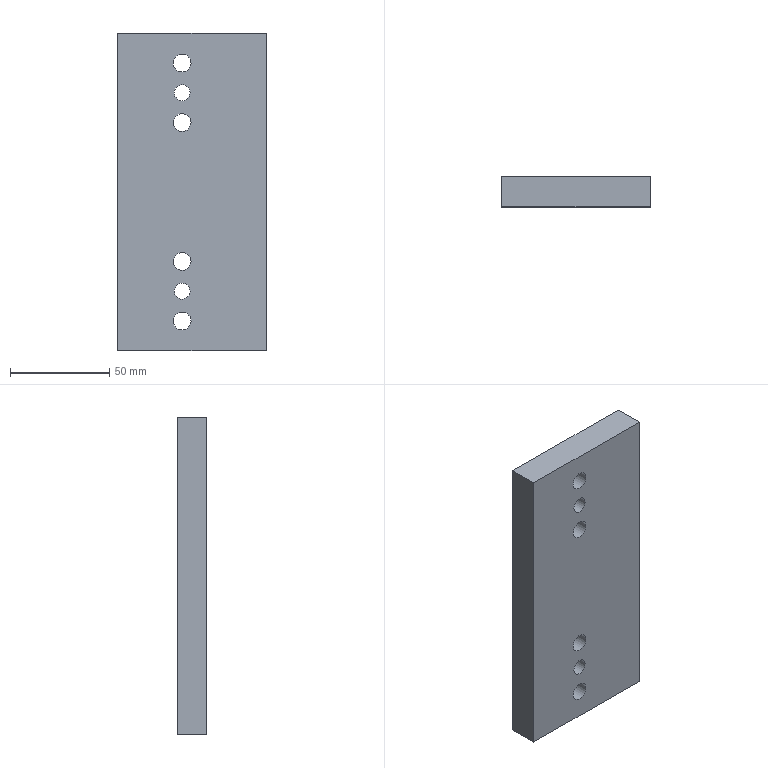Part | STEP file | SN10_008_007-02_PLACA | 1 solid | 12 faces | box 75 x 15 x 160 mm | volume 174675 mm3 | cylinder 6 | plane 6 | commonest cylinder face diameters 9 x4 8 x2
STEP:
#1=CARTESIAN_POINT('',(0.,0.,0.));
#2=DIRECTION('',(0.,0.,1.));
#3=DIRECTION('',(1.,0.,0.));
#4=AXIS2_PLACEMENT_3D('',#1,#2,#3);
#5=CARTESIAN_POINT('',(279.639,240.,404.352));
#6=VERTEX_POINT('',#5);
#7=CARTESIAN_POINT('',(276.129,240.,406.27));
#8=DIRECTION('',(0.,-1.,0.));
#9=DIRECTION('',(1.,0.,0.));
#10=AXIS2_PLACEMENT_3D('',#7,#8,#9);
#11=CIRCLE('',#10,4.);
#12=CARTESIAN_POINT('',(276.129,240.1,406.27));
#13=DIRECTION('',(0.,1.,0.));
#14=DIRECTION('',(0.8776,0.,-0.4794));
#15=AXIS2_PLACEMENT_3D('',#12,#13,#14);
#16=CYLINDRICAL_SURFACE('',#15,4.);
#17=CARTESIAN_POINT('',(12.066,-0.1));
#18=DIRECTION('',(-1.,0.));
#19=VECTOR('',#18,1.);
#20=LINE('',#17,#19);
#21=(GEOMETRIC_REPRESENTATION_CONTEXT(2)PARAMETRIC_REPRESENTATION_CONTEXT()REPRESENTATION_CONTEXT('',''));
#22=DEFINITIONAL_REPRESENTATION('',(#20),#21);
#23=PCURVE('',#16,#22);
#24=CARTESIAN_POINT('',(318.629,240.,446.));
#25=DIRECTION('',(0.,-1.,0.));
#26=DIRECTION('',(0.,0.,-1.));
#27=AXIS2_PLACEMENT_3D('',#24,#25,#26);
#28=PLANE('',#27);
#29=CARTESIAN_POINT('',(39.73,-42.5));
#30=DIRECTION('',(0.,1.));
#31=AXIS2_PLACEMENT_2D('',#29,#30);
#32=CIRCLE('',#31,4.);
#33=(GEOMETRIC_REPRESENTATION_CONTEXT(2)PARAMETRIC_REPRESENTATION_CONTEXT()REPRESENTATION_CONTEXT('',''));
#34=DEFINITIONAL_REPRESENTATION('',(#32),#33);
#35=PCURVE('',#28,#34);
#36=SURFACE_CURVE('',#11,(#23,#35),.PCURVE_S1.);
#37=EDGE_CURVE('',#6,#6,#36,.T.);
#38=ORIENTED_EDGE('',*,*,#37,.F.);
#39=CARTESIAN_POINT('',(279.639,255.,404.352));
#40=VERTEX_POINT('',#39);
#41=CARTESIAN_POINT('',(279.639,240.,404.352));
#42=CARTESIAN_POINT('',(279.639,255.,404.352));
#43=B_SPLINE_CURVE_WITH_KNOTS('',1,(#41,#42),.UNSPECIFIED.,.F.,.F.,(2,2),(-0.1,14.9),.PIECEWISE_BEZIER_KNOTS.);
#44=CARTESIAN_POINT('',(6.283,0.));
#45=DIRECTION('',(0.,1.));
#46=VECTOR('',#45,1.);
#47=LINE('',#44,#46);
#48=(GEOMETRIC_REPRESENTATION_CONTEXT(2)PARAMETRIC_REPRESENTATION_CONTEXT()REPRESENTATION_CONTEXT('',''));
#49=DEFINITIONAL_REPRESENTATION('',(#47),#48);
#50=PCURVE('',#16,#49);
#51=CARTESIAN_POINT('',(0.,0.));
#52=DIRECTION('',(0.,1.));
#53=VECTOR('',#52,1.);
#54=LINE('',#51,#53);
#55=(GEOMETRIC_REPRESENTATION_CONTEXT(2)PARAMETRIC_REPRESENTATION_CONTEXT()REPRESENTATION_CONTEXT('',''));
#56=DEFINITIONAL_REPRESENTATION('',(#54),#55);
#57=PCURVE('',#16,#56);
#58=SEAM_CURVE('',#43,(#50,#57),.PCURVE_S1.);
#59=EDGE_CURVE('',#6,#40,#58,.T.);
#60=ORIENTED_EDGE('',*,*,#59,.T.);
#61=CARTESIAN_POINT('',(276.129,255.,406.27));
#62=DIRECTION('',(0.,1.,0.));
#63=DIRECTION('',(1.,0.,0.));
#64=AXIS2_PLACEMENT_3D('',#61,#62,#63);
#65=CIRCLE('',#64,4.);
#66=CARTESIAN_POINT('',(-0.5,14.9));
#67=DIRECTION('',(1.,0.));
#68=VECTOR('',#67,1.);
#69=LINE('',#66,#68);
#70=(GEOMETRIC_REPRESENTATION_CONTEXT(2)PARAMETRIC_REPRESENTATION_CONTEXT()REPRESENTATION_CONTEXT('',''));
#71=DEFINITIONAL_REPRESENTATION('',(#69),#70);
#72=PCURVE('',#16,#71);
#73=CARTESIAN_POINT('',(243.629,255.,446.));
#74=DIRECTION('',(0.,1.,0.));
#75=DIRECTION('',(0.,0.,1.));
#76=AXIS2_PLACEMENT_3D('',#73,#74,#75);
#77=PLANE('',#76);
#78=CARTESIAN_POINT('',(-39.73,32.5));
#79=DIRECTION('',(0.,1.));
#80=AXIS2_PLACEMENT_2D('',#78,#79);
#81=CIRCLE('',#80,4.);
#82=(GEOMETRIC_REPRESENTATION_CONTEXT(2)PARAMETRIC_REPRESENTATION_CONTEXT()REPRESENTATION_CONTEXT('',''));
#83=DEFINITIONAL_REPRESENTATION('',(#81),#82);
#84=PCURVE('',#77,#83);
#85=SURFACE_CURVE('',#65,(#72,#84),.PCURVE_S1.);
#86=EDGE_CURVE('',#40,#40,#85,.T.);
#87=ORIENTED_EDGE('',*,*,#86,.F.);
#88=ORIENTED_EDGE('',*,*,#59,.F.);
#89=EDGE_LOOP('',(#38,#60,#87,#88));
#90=FACE_BOUND('',#89,.F.);
#91=ADVANCED_FACE('',(#90),#16,.F.);
#92=CARTESIAN_POINT('',(243.629,240.,436.27));
#93=VERTEX_POINT('',#92);
#94=CARTESIAN_POINT('',(243.629,240.,276.27));
#95=VERTEX_POINT('',#94);
#96=CARTESIAN_POINT('',(243.629,240.,436.27));
#97=DIRECTION('',(0.,0.,-1.));
#98=VECTOR('',#97,1.);
#99=LINE('',#96,#98);
#100=CARTESIAN_POINT('',(9.73,-75.));
#101=DIRECTION('',(1.,0.));
#102=VECTOR('',#101,1.);
#103=LINE('',#100,#102);
#104=(GEOMETRIC_REPRESENTATION_CONTEXT(2)PARAMETRIC_REPRESENTATION_CONTEXT()REPRESENTATION_CONTEXT('',''));
#105=DEFINITIONAL_REPRESENTATION('',(#103),#104);
#106=PCURVE('',#28,#105);
#107=CARTESIAN_POINT('',(243.629,255.,446.));
#108=DIRECTION('',(1.,0.,0.));
#109=DIRECTION('',(0.,0.,-1.));
#110=AXIS2_PLACEMENT_3D('',#107,#108,#109);
#111=PLANE('',#110);
#112=CARTESIAN_POINT('',(9.73,-15.));
#113=DIRECTION('',(1.,0.));
#114=VECTOR('',#113,1.);
#115=LINE('',#112,#114);
#116=(GEOMETRIC_REPRESENTATION_CONTEXT(2)PARAMETRIC_REPRESENTATION_CONTEXT()REPRESENTATION_CONTEXT('',''));
#117=DEFINITIONAL_REPRESENTATION('',(#115),#116);
#118=PCURVE('',#111,#117);
#119=SURFACE_CURVE('',#99,(#106,#118),.PCURVE_S1.);
#120=EDGE_CURVE('',#93,#95,#119,.T.);
#121=ORIENTED_EDGE('',*,*,#120,.T.);
#122=CARTESIAN_POINT('',(318.629,240.,276.27));
#123=VERTEX_POINT('',#122);
#124=CARTESIAN_POINT('',(318.629,240.,276.27));
#125=DIRECTION('',(-1.,0.,0.));
#126=VECTOR('',#125,1.);
#127=LINE('',#124,#126);
#128=CARTESIAN_POINT('',(169.73,0.));
#129=DIRECTION('',(0.,-1.));
#130=VECTOR('',#129,1.);
#131=LINE('',#128,#130);
#132=(GEOMETRIC_REPRESENTATION_CONTEXT(2)PARAMETRIC_REPRESENTATION_CONTEXT()REPRESENTATION_CONTEXT('',''));
#133=DEFINITIONAL_REPRESENTATION('',(#131),#132);
#134=PCURVE('',#28,#133);
#135=CARTESIAN_POINT('',(243.629,270.,276.27));
#136=DIRECTION('',(0.,0.,-1.));
#137=DIRECTION('',(-1.,0.,0.));
#138=AXIS2_PLACEMENT_3D('',#135,#136,#137);
#139=PLANE('',#138);
#140=CARTESIAN_POINT('',(-75.,-30.));
#141=DIRECTION('',(1.,0.));
#142=VECTOR('',#141,1.);
#143=LINE('',#140,#142);
#144=(GEOMETRIC_REPRESENTATION_CONTEXT(2)PARAMETRIC_REPRESENTATION_CONTEXT()REPRESENTATION_CONTEXT('',''));
#145=DEFINITIONAL_REPRESENTATION('',(#143),#144);
#146=PCURVE('',#139,#145);
#147=SURFACE_CURVE('',#127,(#134,#146),.PCURVE_S1.);
#148=EDGE_CURVE('',#123,#95,#147,.T.);
#149=ORIENTED_EDGE('',*,*,#148,.F.);
#150=CARTESIAN_POINT('',(318.629,240.,436.27));
#151=VERTEX_POINT('',#150);
#152=CARTESIAN_POINT('',(318.629,240.,436.27));
#153=DIRECTION('',(0.,0.,-1.));
#154=VECTOR('',#153,1.);
#155=LINE('',#152,#154);
#156=CARTESIAN_POINT('',(9.73,0.));
#157=DIRECTION('',(1.,0.));
#158=VECTOR('',#157,1.);
#159=LINE('',#156,#158);
#160=(GEOMETRIC_REPRESENTATION_CONTEXT(2)PARAMETRIC_REPRESENTATION_CONTEXT()REPRESENTATION_CONTEXT('',''));
#161=DEFINITIONAL_REPRESENTATION('',(#159),#160);
#162=PCURVE('',#28,#161);
#163=CARTESIAN_POINT('',(318.629,240.,446.));
#164=DIRECTION('',(-1.,0.,0.));
#165=DIRECTION('',(0.,0.,1.));
#166=AXIS2_PLACEMENT_3D('',#163,#164,#165);
#167=PLANE('',#166);
#168=CARTESIAN_POINT('',(-9.73,0.));
#169=DIRECTION('',(-1.,0.));
#170=VECTOR('',#169,1.);
#171=LINE('',#168,#170);
#172=(GEOMETRIC_REPRESENTATION_CONTEXT(2)PARAMETRIC_REPRESENTATION_CONTEXT()REPRESENTATION_CONTEXT('',''));
#173=DEFINITIONAL_REPRESENTATION('',(#171),#172);
#174=PCURVE('',#167,#173);
#175=SURFACE_CURVE('',#155,(#162,#174),.PCURVE_S1.);
#176=EDGE_CURVE('',#151,#123,#175,.T.);
#177=ORIENTED_EDGE('',*,*,#176,.F.);
#178=CARTESIAN_POINT('',(243.629,240.,436.27));
#179=DIRECTION('',(1.,0.,0.));
#180=VECTOR('',#179,1.);
#181=LINE('',#178,#180);
#182=CARTESIAN_POINT('',(9.73,-75.));
#183=DIRECTION('',(0.,1.));
#184=VECTOR('',#183,1.);
#185=LINE('',#182,#184);
#186=(GEOMETRIC_REPRESENTATION_CONTEXT(2)PARAMETRIC_REPRESENTATION_CONTEXT()REPRESENTATION_CONTEXT('',''));
#187=DEFINITIONAL_REPRESENTATION('',(#185),#186);
#188=PCURVE('',#28,#187);
#189=CARTESIAN_POINT('',(243.629,255.,436.27));
#190=DIRECTION('',(0.,0.,1.));
#191=DIRECTION('',(1.,0.,0.));
#192=AXIS2_PLACEMENT_3D('',#189,#190,#191);
#193=PLANE('',#192);
#194=CARTESIAN_POINT('',(0.,-15.));
#195=DIRECTION('',(1.,0.));
#196=VECTOR('',#195,1.);
#197=LINE('',#194,#196);
#198=(GEOMETRIC_REPRESENTATION_CONTEXT(2)PARAMETRIC_REPRESENTATION_CONTEXT()REPRESENTATION_CONTEXT('',''));
#199=DEFINITIONAL_REPRESENTATION('',(#197),#198);
#200=PCURVE('',#193,#199);
#201=SURFACE_CURVE('',#181,(#188,#200),.PCURVE_S1.);
#202=EDGE_CURVE('',#93,#151,#201,.T.);
#203=ORIENTED_EDGE('',*,*,#202,.F.);
#204=EDGE_LOOP('',(#121,#149,#177,#203));
#205=FACE_BOUND('',#204,.T.);
#206=ORIENTED_EDGE('',*,*,#37,.F.);
#207=EDGE_LOOP('',(#206));
#208=FACE_BOUND('',#207,.T.);
#209=CARTESIAN_POINT('',(279.639,240.,304.352));
#210=VERTEX_POINT('',#209);
#211=CARTESIAN_POINT('',(276.129,240.,306.27));
#212=DIRECTION('',(0.,-1.,0.));
#213=DIRECTION('',(1.,0.,0.));
#214=AXIS2_PLACEMENT_3D('',#211,#212,#213);
#215=CIRCLE('',#214,4.);
#216=CARTESIAN_POINT('',(139.73,-42.5));
#217=DIRECTION('',(0.,1.));
#218=AXIS2_PLACEMENT_2D('',#216,#217);
#219=CIRCLE('',#218,4.);
#220=(GEOMETRIC_REPRESENTATION_CONTEXT(2)PARAMETRIC_REPRESENTATION_CONTEXT()REPRESENTATION_CONTEXT('',''));
#221=DEFINITIONAL_REPRESENTATION('',(#219),#220);
#222=PCURVE('',#28,#221);
#223=CARTESIAN_POINT('',(276.129,240.1,306.27));
#224=DIRECTION('',(0.,1.,0.));
#225=DIRECTION('',(0.8776,0.,-0.4794));
#226=AXIS2_PLACEMENT_3D('',#223,#224,#225);
#227=CYLINDRICAL_SURFACE('',#226,4.);
#228=CARTESIAN_POINT('',(12.066,-0.1));
#229=DIRECTION('',(-1.,0.));
#230=VECTOR('',#229,1.);
#231=LINE('',#228,#230);
#232=(GEOMETRIC_REPRESENTATION_CONTEXT(2)PARAMETRIC_REPRESENTATION_CONTEXT()REPRESENTATION_CONTEXT('',''));
#233=DEFINITIONAL_REPRESENTATION('',(#231),#232);
#234=PCURVE('',#227,#233);
#235=SURFACE_CURVE('',#215,(#222,#234),.PCURVE_S1.);
#236=EDGE_CURVE('',#210,#210,#235,.T.);
#237=ORIENTED_EDGE('',*,*,#236,.F.);
#238=EDGE_LOOP('',(#237));
#239=FACE_BOUND('',#238,.T.);
#240=CARTESIAN_POINT('',(280.078,240.,319.113));
#241=VERTEX_POINT('',#240);
#242=CARTESIAN_POINT('',(276.129,240.,321.27));
#243=DIRECTION('',(0.,-1.,0.));
#244=DIRECTION('',(1.,0.,0.));
#245=AXIS2_PLACEMENT_3D('',#242,#243,#244);
#246=CIRCLE('',#245,4.5);
#247=CARTESIAN_POINT('',(124.73,-42.5));
#248=DIRECTION('',(0.,1.));
#249=AXIS2_PLACEMENT_2D('',#247,#248);
#250=CIRCLE('',#249,4.5);
#251=(GEOMETRIC_REPRESENTATION_CONTEXT(2)PARAMETRIC_REPRESENTATION_CONTEXT()REPRESENTATION_CONTEXT('',''));
#252=DEFINITIONAL_REPRESENTATION('',(#250),#251);
#253=PCURVE('',#28,#252);
#254=CARTESIAN_POINT('',(276.129,240.1,321.27));
#255=DIRECTION('',(0.,1.,0.));
#256=DIRECTION('',(0.8776,0.,-0.4794));
#257=AXIS2_PLACEMENT_3D('',#254,#255,#256);
#258=CYLINDRICAL_SURFACE('',#257,4.5);
#259=CARTESIAN_POINT('',(12.066,-0.1));
#260=DIRECTION('',(-1.,0.));
#261=VECTOR('',#260,1.);
#262=LINE('',#259,#261);
#263=(GEOMETRIC_REPRESENTATION_CONTEXT(2)PARAMETRIC_REPRESENTATION_CONTEXT()REPRESENTATION_CONTEXT('',''));
#264=DEFINITIONAL_REPRESENTATION('',(#262),#263);
#265=PCURVE('',#258,#264);
#266=SURFACE_CURVE('',#246,(#253,#265),.PCURVE_S1.);
#267=EDGE_CURVE('',#241,#241,#266,.T.);
#268=ORIENTED_EDGE('',*,*,#267,.F.);
#269=EDGE_LOOP('',(#268));
#270=FACE_BOUND('',#269,.T.);
#271=CARTESIAN_POINT('',(280.078,240.,289.113));
#272=VERTEX_POINT('',#271);
#273=CARTESIAN_POINT('',(276.129,240.,291.27));
#274=DIRECTION('',(0.,-1.,0.));
#275=DIRECTION('',(1.,0.,0.));
#276=AXIS2_PLACEMENT_3D('',#273,#274,#275);
#277=CIRCLE('',#276,4.5);
#278=CARTESIAN_POINT('',(154.73,-42.5));
#279=DIRECTION('',(0.,1.));
#280=AXIS2_PLACEMENT_2D('',#278,#279);
#281=CIRCLE('',#280,4.5);
#282=(GEOMETRIC_REPRESENTATION_CONTEXT(2)PARAMETRIC_REPRESENTATION_CONTEXT()REPRESENTATION_CONTEXT('',''));
#283=DEFINITIONAL_REPRESENTATION('',(#281),#282);
#284=PCURVE('',#28,#283);
#285=CARTESIAN_POINT('',(276.129,240.1,291.27));
#286=DIRECTION('',(0.,1.,0.));
#287=DIRECTION('',(0.8776,0.,-0.4794));
#288=AXIS2_PLACEMENT_3D('',#285,#286,#287);
#289=CYLINDRICAL_SURFACE('',#288,4.5);
#290=CARTESIAN_POINT('',(12.066,-0.1));
#291=DIRECTION('',(-1.,0.));
#292=VECTOR('',#291,1.);
#293=LINE('',#290,#292);
#294=(GEOMETRIC_REPRESENTATION_CONTEXT(2)PARAMETRIC_REPRESENTATION_CONTEXT()REPRESENTATION_CONTEXT('',''));
#295=DEFINITIONAL_REPRESENTATION('',(#293),#294);
#296=PCURVE('',#289,#295);
#297=SURFACE_CURVE('',#277,(#284,#296),.PCURVE_S1.);
#298=EDGE_CURVE('',#272,#272,#297,.T.);
#299=ORIENTED_EDGE('',*,*,#298,.F.);
#300=EDGE_LOOP('',(#299));
#301=FACE_BOUND('',#300,.T.);
#302=CARTESIAN_POINT('',(280.078,240.,389.113));
#303=VERTEX_POINT('',#302);
#304=CARTESIAN_POINT('',(276.129,240.,391.27));
#305=DIRECTION('',(0.,-1.,0.));
#306=DIRECTION('',(1.,0.,0.));
#307=AXIS2_PLACEMENT_3D('',#304,#305,#306);
#308=CIRCLE('',#307,4.5);
#309=CARTESIAN_POINT('',(54.73,-42.5));
#310=DIRECTION('',(0.,1.));
#311=AXIS2_PLACEMENT_2D('',#309,#310);
#312=CIRCLE('',#311,4.5);
#313=(GEOMETRIC_REPRESENTATION_CONTEXT(2)PARAMETRIC_REPRESENTATION_CONTEXT()REPRESENTATION_CONTEXT('',''));
#314=DEFINITIONAL_REPRESENTATION('',(#312),#313);
#315=PCURVE('',#28,#314);
#316=CARTESIAN_POINT('',(276.129,240.1,391.27));
#317=DIRECTION('',(0.,1.,0.));
#318=DIRECTION('',(0.8776,0.,-0.4794));
#319=AXIS2_PLACEMENT_3D('',#316,#317,#318);
#320=CYLINDRICAL_SURFACE('',#319,4.5);
#321=CARTESIAN_POINT('',(12.066,-0.1));
#322=DIRECTION('',(-1.,0.));
#323=VECTOR('',#322,1.);
#324=LINE('',#321,#323);
#325=(GEOMETRIC_REPRESENTATION_CONTEXT(2)PARAMETRIC_REPRESENTATION_CONTEXT()REPRESENTATION_CONTEXT('',''));
#326=DEFINITIONAL_REPRESENTATION('',(#324),#325);
#327=PCURVE('',#320,#326);
#328=SURFACE_CURVE('',#308,(#315,#327),.PCURVE_S1.);
#329=EDGE_CURVE('',#303,#303,#328,.T.);
#330=ORIENTED_EDGE('',*,*,#329,.F.);
#331=EDGE_LOOP('',(#330));
#332=FACE_BOUND('',#331,.T.);
#333=CARTESIAN_POINT('',(280.078,240.,419.113));
#334=VERTEX_POINT('',#333);
#335=CARTESIAN_POINT('',(276.129,240.,421.27));
#336=DIRECTION('',(0.,-1.,0.));
#337=DIRECTION('',(1.,0.,0.));
#338=AXIS2_PLACEMENT_3D('',#335,#336,#337);
#339=CIRCLE('',#338,4.5);
#340=CARTESIAN_POINT('',(24.73,-42.5));
#341=DIRECTION('',(0.,1.));
#342=AXIS2_PLACEMENT_2D('',#340,#341);
#343=CIRCLE('',#342,4.5);
#344=(GEOMETRIC_REPRESENTATION_CONTEXT(2)PARAMETRIC_REPRESENTATION_CONTEXT()REPRESENTATION_CONTEXT('',''));
#345=DEFINITIONAL_REPRESENTATION('',(#343),#344);
#346=PCURVE('',#28,#345);
#347=CARTESIAN_POINT('',(276.129,240.1,421.27));
#348=DIRECTION('',(0.,1.,0.));
#349=DIRECTION('',(0.8776,0.,-0.4794));
#350=AXIS2_PLACEMENT_3D('',#347,#348,#349);
#351=CYLINDRICAL_SURFACE('',#350,4.5);
#352=CARTESIAN_POINT('',(12.066,-0.1));
#353=DIRECTION('',(-1.,0.));
#354=VECTOR('',#353,1.);
#355=LINE('',#352,#354);
#356=(GEOMETRIC_REPRESENTATION_CONTEXT(2)PARAMETRIC_REPRESENTATION_CONTEXT()REPRESENTATION_CONTEXT('',''));
#357=DEFINITIONAL_REPRESENTATION('',(#355),#356);
#358=PCURVE('',#351,#357);
#359=SURFACE_CURVE('',#339,(#346,#358),.PCURVE_S1.);
#360=EDGE_CURVE('',#334,#334,#359,.T.);
#361=ORIENTED_EDGE('',*,*,#360,.F.);
#362=EDGE_LOOP('',(#361));
#363=FACE_BOUND('',#362,.T.);
#364=ADVANCED_FACE('',(#205,#208,#239,#270,#301,#332,#363),#28,.T.);
#365=CARTESIAN_POINT('',(318.629,255.,436.27));
#366=VERTEX_POINT('',#365);
#367=CARTESIAN_POINT('',(318.629,255.,276.27));
#368=VERTEX_POINT('',#367);
#369=CARTESIAN_POINT('',(318.629,255.,436.27));
#370=DIRECTION('',(0.,0.,-1.));
#371=VECTOR('',#370,1.);
#372=LINE('',#369,#371);
#373=CARTESIAN_POINT('',(-9.73,75.));
#374=DIRECTION('',(-1.,0.));
#375=VECTOR('',#374,1.);
#376=LINE('',#373,#375);
#377=(GEOMETRIC_REPRESENTATION_CONTEXT(2)PARAMETRIC_REPRESENTATION_CONTEXT()REPRESENTATION_CONTEXT('',''));
#378=DEFINITIONAL_REPRESENTATION('',(#376),#377);
#379=PCURVE('',#77,#378);
#380=CARTESIAN_POINT('',(-9.73,15.));
#381=DIRECTION('',(-1.,0.));
#382=VECTOR('',#381,1.);
#383=LINE('',#380,#382);
#384=(GEOMETRIC_REPRESENTATION_CONTEXT(2)PARAMETRIC_REPRESENTATION_CONTEXT()REPRESENTATION_CONTEXT('',''));
#385=DEFINITIONAL_REPRESENTATION('',(#383),#384);
#386=PCURVE('',#167,#385);
#387=SURFACE_CURVE('',#372,(#379,#386),.PCURVE_S1.);
#388=EDGE_CURVE('',#366,#368,#387,.T.);
#389=ORIENTED_EDGE('',*,*,#388,.T.);
#390=CARTESIAN_POINT('',(243.629,255.,276.27));
#391=VERTEX_POINT('',#390);
#392=CARTESIAN_POINT('',(243.629,255.,276.27));
#393=DIRECTION('',(1.,0.,0.));
#394=VECTOR('',#393,1.);
#395=LINE('',#392,#394);
#396=CARTESIAN_POINT('',(-169.73,0.));
#397=DIRECTION('',(0.,1.));
#398=VECTOR('',#397,1.);
#399=LINE('',#396,#398);
#400=(GEOMETRIC_REPRESENTATION_CONTEXT(2)PARAMETRIC_REPRESENTATION_CONTEXT()REPRESENTATION_CONTEXT('',''));
#401=DEFINITIONAL_REPRESENTATION('',(#399),#400);
#402=PCURVE('',#77,#401);
#403=CARTESIAN_POINT('',(0.,-15.));
#404=DIRECTION('',(-1.,0.));
#405=VECTOR('',#404,1.);
#406=LINE('',#403,#405);
#407=(GEOMETRIC_REPRESENTATION_CONTEXT(2)PARAMETRIC_REPRESENTATION_CONTEXT()REPRESENTATION_CONTEXT('',''));
#408=DEFINITIONAL_REPRESENTATION('',(#406),#407);
#409=PCURVE('',#139,#408);
#410=SURFACE_CURVE('',#395,(#402,#409),.PCURVE_S1.);
#411=EDGE_CURVE('',#391,#368,#410,.T.);
#412=ORIENTED_EDGE('',*,*,#411,.F.);
#413=CARTESIAN_POINT('',(243.629,255.,436.27));
#414=VERTEX_POINT('',#413);
#415=CARTESIAN_POINT('',(243.629,255.,436.27));
#416=DIRECTION('',(0.,0.,-1.));
#417=VECTOR('',#416,1.);
#418=LINE('',#415,#417);
#419=CARTESIAN_POINT('',(-9.73,0.));
#420=DIRECTION('',(-1.,0.));
#421=VECTOR('',#420,1.);
#422=LINE('',#419,#421);
#423=(GEOMETRIC_REPRESENTATION_CONTEXT(2)PARAMETRIC_REPRESENTATION_CONTEXT()REPRESENTATION_CONTEXT('',''));
#424=DEFINITIONAL_REPRESENTATION('',(#422),#423);
#425=PCURVE('',#77,#424);
#426=CARTESIAN_POINT('',(9.73,0.));
#427=DIRECTION('',(1.,0.));
#428=VECTOR('',#427,1.);
#429=LINE('',#426,#428);
#430=(GEOMETRIC_REPRESENTATION_CONTEXT(2)PARAMETRIC_REPRESENTATION_CONTEXT()REPRESENTATION_CONTEXT('',''));
#431=DEFINITIONAL_REPRESENTATION('',(#429),#430);
#432=PCURVE('',#111,#431);
#433=SURFACE_CURVE('',#418,(#425,#432),.PCURVE_S1.);
#434=EDGE_CURVE('',#414,#391,#433,.T.);
#435=ORIENTED_EDGE('',*,*,#434,.F.);
#436=CARTESIAN_POINT('',(243.629,255.,436.27));
#437=DIRECTION('',(1.,0.,0.));
#438=VECTOR('',#437,1.);
#439=LINE('',#436,#438);
#440=CARTESIAN_POINT('',(-9.73,0.));
#441=DIRECTION('',(0.,1.));
#442=VECTOR('',#441,1.);
#443=LINE('',#440,#442);
#444=(GEOMETRIC_REPRESENTATION_CONTEXT(2)PARAMETRIC_REPRESENTATION_CONTEXT()REPRESENTATION_CONTEXT('',''));
#445=DEFINITIONAL_REPRESENTATION('',(#443),#444);
#446=PCURVE('',#77,#445);
#447=CARTESIAN_POINT('',(0.,0.));
#448=DIRECTION('',(1.,0.));
#449=VECTOR('',#448,1.);
#450=LINE('',#447,#449);
#451=(GEOMETRIC_REPRESENTATION_CONTEXT(2)PARAMETRIC_REPRESENTATION_CONTEXT()REPRESENTATION_CONTEXT('',''));
#452=DEFINITIONAL_REPRESENTATION('',(#450),#451);
#453=PCURVE('',#193,#452);
#454=SURFACE_CURVE('',#439,(#446,#453),.PCURVE_S1.);
#455=EDGE_CURVE('',#414,#366,#454,.T.);
#456=ORIENTED_EDGE('',*,*,#455,.T.);
#457=EDGE_LOOP('',(#389,#412,#435,#456));
#458=FACE_BOUND('',#457,.T.);
#459=ORIENTED_EDGE('',*,*,#86,.F.);
#460=EDGE_LOOP('',(#459));
#461=FACE_BOUND('',#460,.T.);
#462=CARTESIAN_POINT('',(279.639,255.,304.352));
#463=VERTEX_POINT('',#462);
#464=CARTESIAN_POINT('',(276.129,255.,306.27));
#465=DIRECTION('',(0.,1.,0.));
#466=DIRECTION('',(1.,0.,0.));
#467=AXIS2_PLACEMENT_3D('',#464,#465,#466);
#468=CIRCLE('',#467,4.);
#469=CARTESIAN_POINT('',(-139.73,32.5));
#470=DIRECTION('',(0.,1.));
#471=AXIS2_PLACEMENT_2D('',#469,#470);
#472=CIRCLE('',#471,4.);
#473=(GEOMETRIC_REPRESENTATION_CONTEXT(2)PARAMETRIC_REPRESENTATION_CONTEXT()REPRESENTATION_CONTEXT('',''));
#474=DEFINITIONAL_REPRESENTATION('',(#472),#473);
#475=PCURVE('',#77,#474);
#476=CARTESIAN_POINT('',(-0.5,14.9));
#477=DIRECTION('',(1.,0.));
#478=VECTOR('',#477,1.);
#479=LINE('',#476,#478);
#480=(GEOMETRIC_REPRESENTATION_CONTEXT(2)PARAMETRIC_REPRESENTATION_CONTEXT()REPRESENTATION_CONTEXT('',''));
#481=DEFINITIONAL_REPRESENTATION('',(#479),#480);
#482=PCURVE('',#227,#481);
#483=SURFACE_CURVE('',#468,(#475,#482),.PCURVE_S1.);
#484=EDGE_CURVE('',#463,#463,#483,.T.);
#485=ORIENTED_EDGE('',*,*,#484,.F.);
#486=EDGE_LOOP('',(#485));
#487=FACE_BOUND('',#486,.T.);
#488=CARTESIAN_POINT('',(280.078,255.,319.113));
#489=VERTEX_POINT('',#488);
#490=CARTESIAN_POINT('',(276.129,255.,321.27));
#491=DIRECTION('',(0.,1.,0.));
#492=DIRECTION('',(1.,0.,0.));
#493=AXIS2_PLACEMENT_3D('',#490,#491,#492);
#494=CIRCLE('',#493,4.5);
#495=CARTESIAN_POINT('',(-124.73,32.5));
#496=DIRECTION('',(0.,1.));
#497=AXIS2_PLACEMENT_2D('',#495,#496);
#498=CIRCLE('',#497,4.5);
#499=(GEOMETRIC_REPRESENTATION_CONTEXT(2)PARAMETRIC_REPRESENTATION_CONTEXT()REPRESENTATION_CONTEXT('',''));
#500=DEFINITIONAL_REPRESENTATION('',(#498),#499);
#501=PCURVE('',#77,#500);
#502=CARTESIAN_POINT('',(-0.5,14.9));
#503=DIRECTION('',(1.,0.));
#504=VECTOR('',#503,1.);
#505=LINE('',#502,#504);
#506=(GEOMETRIC_REPRESENTATION_CONTEXT(2)PARAMETRIC_REPRESENTATION_CONTEXT()REPRESENTATION_CONTEXT('',''));
#507=DEFINITIONAL_REPRESENTATION('',(#505),#506);
#508=PCURVE('',#258,#507);
#509=SURFACE_CURVE('',#494,(#501,#508),.PCURVE_S1.);
#510=EDGE_CURVE('',#489,#489,#509,.T.);
#511=ORIENTED_EDGE('',*,*,#510,.F.);
#512=EDGE_LOOP('',(#511));
#513=FACE_BOUND('',#512,.T.);
#514=CARTESIAN_POINT('',(280.078,255.,289.113));
#515=VERTEX_POINT('',#514);
#516=CARTESIAN_POINT('',(276.129,255.,291.27));
#517=DIRECTION('',(0.,1.,0.));
#518=DIRECTION('',(1.,0.,0.));
#519=AXIS2_PLACEMENT_3D('',#516,#517,#518);
#520=CIRCLE('',#519,4.5);
#521=CARTESIAN_POINT('',(-154.73,32.5));
#522=DIRECTION('',(0.,1.));
#523=AXIS2_PLACEMENT_2D('',#521,#522);
#524=CIRCLE('',#523,4.5);
#525=(GEOMETRIC_REPRESENTATION_CONTEXT(2)PARAMETRIC_REPRESENTATION_CONTEXT()REPRESENTATION_CONTEXT('',''));
#526=DEFINITIONAL_REPRESENTATION('',(#524),#525);
#527=PCURVE('',#77,#526);
#528=CARTESIAN_POINT('',(-0.5,14.9));
#529=DIRECTION('',(1.,0.));
#530=VECTOR('',#529,1.);
#531=LINE('',#528,#530);
#532=(GEOMETRIC_REPRESENTATION_CONTEXT(2)PARAMETRIC_REPRESENTATION_CONTEXT()REPRESENTATION_CONTEXT('',''));
#533=DEFINITIONAL_REPRESENTATION('',(#531),#532);
#534=PCURVE('',#289,#533);
#535=SURFACE_CURVE('',#520,(#527,#534),.PCURVE_S1.);
#536=EDGE_CURVE('',#515,#515,#535,.T.);
#537=ORIENTED_EDGE('',*,*,#536,.F.);
#538=EDGE_LOOP('',(#537));
#539=FACE_BOUND('',#538,.T.);
#540=CARTESIAN_POINT('',(280.078,255.,389.113));
#541=VERTEX_POINT('',#540);
#542=CARTESIAN_POINT('',(276.129,255.,391.27));
#543=DIRECTION('',(0.,1.,0.));
#544=DIRECTION('',(1.,0.,0.));
#545=AXIS2_PLACEMENT_3D('',#542,#543,#544);
#546=CIRCLE('',#545,4.5);
#547=CARTESIAN_POINT('',(-54.73,32.5));
#548=DIRECTION('',(0.,1.));
#549=AXIS2_PLACEMENT_2D('',#547,#548);
#550=CIRCLE('',#549,4.5);
#551=(GEOMETRIC_REPRESENTATION_CONTEXT(2)PARAMETRIC_REPRESENTATION_CONTEXT()REPRESENTATION_CONTEXT('',''));
#552=DEFINITIONAL_REPRESENTATION('',(#550),#551);
#553=PCURVE('',#77,#552);
#554=CARTESIAN_POINT('',(-0.5,14.9));
#555=DIRECTION('',(1.,0.));
#556=VECTOR('',#555,1.);
#557=LINE('',#554,#556);
#558=(GEOMETRIC_REPRESENTATION_CONTEXT(2)PARAMETRIC_REPRESENTATION_CONTEXT()REPRESENTATION_CONTEXT('',''));
#559=DEFINITIONAL_REPRESENTATION('',(#557),#558);
#560=PCURVE('',#320,#559);
#561=SURFACE_CURVE('',#546,(#553,#560),.PCURVE_S1.);
#562=EDGE_CURVE('',#541,#541,#561,.T.);
#563=ORIENTED_EDGE('',*,*,#562,.F.);
#564=EDGE_LOOP('',(#563));
#565=FACE_BOUND('',#564,.T.);
#566=CARTESIAN_POINT('',(280.078,255.,419.113));
#567=VERTEX_POINT('',#566);
#568=CARTESIAN_POINT('',(276.129,255.,421.27));
#569=DIRECTION('',(0.,1.,0.));
#570=DIRECTION('',(1.,0.,0.));
#571=AXIS2_PLACEMENT_3D('',#568,#569,#570);
#572=CIRCLE('',#571,4.5);
#573=CARTESIAN_POINT('',(-24.73,32.5));
#574=DIRECTION('',(0.,1.));
#575=AXIS2_PLACEMENT_2D('',#573,#574);
#576=CIRCLE('',#575,4.5);
#577=(GEOMETRIC_REPRESENTATION_CONTEXT(2)PARAMETRIC_REPRESENTATION_CONTEXT()REPRESENTATION_CONTEXT('',''));
#578=DEFINITIONAL_REPRESENTATION('',(#576),#577);
#579=PCURVE('',#77,#578);
#580=CARTESIAN_POINT('',(-0.5,14.9));
#581=DIRECTION('',(1.,0.));
#582=VECTOR('',#581,1.);
#583=LINE('',#580,#582);
#584=(GEOMETRIC_REPRESENTATION_CONTEXT(2)PARAMETRIC_REPRESENTATION_CONTEXT()REPRESENTATION_CONTEXT('',''));
#585=DEFINITIONAL_REPRESENTATION('',(#583),#584);
#586=PCURVE('',#351,#585);
#587=SURFACE_CURVE('',#572,(#579,#586),.PCURVE_S1.);
#588=EDGE_CURVE('',#567,#567,#587,.T.);
#589=ORIENTED_EDGE('',*,*,#588,.F.);
#590=EDGE_LOOP('',(#589));
#591=FACE_BOUND('',#590,.T.);
#592=ADVANCED_FACE('',(#458,#461,#487,#513,#539,#565,#591),#77,.T.);
#593=CARTESIAN_POINT('',(243.629,255.,436.27));
#594=DIRECTION('',(0.,-1.,0.));
#595=VECTOR('',#594,1.);
#596=LINE('',#593,#595);
#597=CARTESIAN_POINT('',(9.73,0.));
#598=DIRECTION('',(0.,-1.));
#599=VECTOR('',#598,1.);
#600=LINE('',#597,#599);
#601=(GEOMETRIC_REPRESENTATION_CONTEXT(2)PARAMETRIC_REPRESENTATION_CONTEXT()REPRESENTATION_CONTEXT('',''));
#602=DEFINITIONAL_REPRESENTATION('',(#600),#601);
#603=PCURVE('',#111,#602);
#604=CARTESIAN_POINT('',(0.,0.));
#605=DIRECTION('',(0.,-1.));
#606=VECTOR('',#605,1.);
#607=LINE('',#604,#606);
#608=(GEOMETRIC_REPRESENTATION_CONTEXT(2)PARAMETRIC_REPRESENTATION_CONTEXT()REPRESENTATION_CONTEXT('',''));
#609=DEFINITIONAL_REPRESENTATION('',(#607),#608);
#610=PCURVE('',#193,#609);
#611=SURFACE_CURVE('',#596,(#603,#610),.PCURVE_S1.);
#612=EDGE_CURVE('',#414,#93,#611,.T.);
#613=ORIENTED_EDGE('',*,*,#612,.F.);
#614=ORIENTED_EDGE('',*,*,#434,.T.);
#615=CARTESIAN_POINT('',(243.629,255.,276.27));
#616=DIRECTION('',(0.,-1.,0.));
#617=VECTOR('',#616,1.);
#618=LINE('',#615,#617);
#619=CARTESIAN_POINT('',(169.73,0.));
#620=DIRECTION('',(0.,-1.));
#621=VECTOR('',#620,1.);
#622=LINE('',#619,#621);
#623=(GEOMETRIC_REPRESENTATION_CONTEXT(2)PARAMETRIC_REPRESENTATION_CONTEXT()REPRESENTATION_CONTEXT('',''));
#624=DEFINITIONAL_REPRESENTATION('',(#622),#623);
#625=PCURVE('',#111,#624);
#626=CARTESIAN_POINT('',(0.,-15.));
#627=DIRECTION('',(0.,-1.));
#628=VECTOR('',#627,1.);
#629=LINE('',#626,#628);
#630=(GEOMETRIC_REPRESENTATION_CONTEXT(2)PARAMETRIC_REPRESENTATION_CONTEXT()REPRESENTATION_CONTEXT('',''));
#631=DEFINITIONAL_REPRESENTATION('',(#629),#630);
#632=PCURVE('',#139,#631);
#633=SURFACE_CURVE('',#618,(#625,#632),.PCURVE_S1.);
#634=EDGE_CURVE('',#391,#95,#633,.T.);
#635=ORIENTED_EDGE('',*,*,#634,.T.);
#636=ORIENTED_EDGE('',*,*,#120,.F.);
#637=EDGE_LOOP('',(#613,#614,#635,#636));
#638=FACE_BOUND('',#637,.T.);
#639=ADVANCED_FACE('',(#638),#111,.F.);
#640=ORIENTED_EDGE('',*,*,#360,.F.);
#641=CARTESIAN_POINT('',(280.078,240.,419.113));
#642=CARTESIAN_POINT('',(280.078,255.,419.113));
#643=B_SPLINE_CURVE_WITH_KNOTS('',1,(#641,#642),.UNSPECIFIED.,.F.,.F.,(2,2),(-0.1,14.9),.PIECEWISE_BEZIER_KNOTS.);
#644=CARTESIAN_POINT('',(6.283,0.));
#645=DIRECTION('',(0.,1.));
#646=VECTOR('',#645,1.);
#647=LINE('',#644,#646);
#648=(GEOMETRIC_REPRESENTATION_CONTEXT(2)PARAMETRIC_REPRESENTATION_CONTEXT()REPRESENTATION_CONTEXT('',''));
#649=DEFINITIONAL_REPRESENTATION('',(#647),#648);
#650=PCURVE('',#351,#649);
#651=CARTESIAN_POINT('',(0.,0.));
#652=DIRECTION('',(0.,1.));
#653=VECTOR('',#652,1.);
#654=LINE('',#651,#653);
#655=(GEOMETRIC_REPRESENTATION_CONTEXT(2)PARAMETRIC_REPRESENTATION_CONTEXT()REPRESENTATION_CONTEXT('',''));
#656=DEFINITIONAL_REPRESENTATION('',(#654),#655);
#657=PCURVE('',#351,#656);
#658=SEAM_CURVE('',#643,(#650,#657),.PCURVE_S1.);
#659=EDGE_CURVE('',#334,#567,#658,.T.);
#660=ORIENTED_EDGE('',*,*,#659,.T.);
#661=ORIENTED_EDGE('',*,*,#588,.F.);
#662=ORIENTED_EDGE('',*,*,#659,.F.);
#663=EDGE_LOOP('',(#640,#660,#661,#662));
#664=FACE_BOUND('',#663,.F.);
#665=ADVANCED_FACE('',(#664),#351,.F.);
#666=ORIENTED_EDGE('',*,*,#329,.F.);
#667=CARTESIAN_POINT('',(280.078,240.,389.113));
#668=CARTESIAN_POINT('',(280.078,255.,389.113));
#669=B_SPLINE_CURVE_WITH_KNOTS('',1,(#667,#668),.UNSPECIFIED.,.F.,.F.,(2,2),(-0.1,14.9),.PIECEWISE_BEZIER_KNOTS.);
#670=CARTESIAN_POINT('',(6.283,0.));
#671=DIRECTION('',(0.,1.));
#672=VECTOR('',#671,1.);
#673=LINE('',#670,#672);
#674=(GEOMETRIC_REPRESENTATION_CONTEXT(2)PARAMETRIC_REPRESENTATION_CONTEXT()REPRESENTATION_CONTEXT('',''));
#675=DEFINITIONAL_REPRESENTATION('',(#673),#674);
#676=PCURVE('',#320,#675);
#677=CARTESIAN_POINT('',(0.,0.));
#678=DIRECTION('',(0.,1.));
#679=VECTOR('',#678,1.);
#680=LINE('',#677,#679);
#681=(GEOMETRIC_REPRESENTATION_CONTEXT(2)PARAMETRIC_REPRESENTATION_CONTEXT()REPRESENTATION_CONTEXT('',''));
#682=DEFINITIONAL_REPRESENTATION('',(#680),#681);
#683=PCURVE('',#320,#682);
#684=SEAM_CURVE('',#669,(#676,#683),.PCURVE_S1.);
#685=EDGE_CURVE('',#303,#541,#684,.T.);
#686=ORIENTED_EDGE('',*,*,#685,.T.);
#687=ORIENTED_EDGE('',*,*,#562,.F.);
#688=ORIENTED_EDGE('',*,*,#685,.F.);
#689=EDGE_LOOP('',(#666,#686,#687,#688));
#690=FACE_BOUND('',#689,.F.);
#691=ADVANCED_FACE('',(#690),#320,.F.);
#692=ORIENTED_EDGE('',*,*,#298,.F.);
#693=CARTESIAN_POINT('',(280.078,240.,289.113));
#694=CARTESIAN_POINT('',(280.078,255.,289.113));
#695=B_SPLINE_CURVE_WITH_KNOTS('',1,(#693,#694),.UNSPECIFIED.,.F.,.F.,(2,2),(-0.1,14.9),.PIECEWISE_BEZIER_KNOTS.);
#696=CARTESIAN_POINT('',(6.283,0.));
#697=DIRECTION('',(0.,1.));
#698=VECTOR('',#697,1.);
#699=LINE('',#696,#698);
#700=(GEOMETRIC_REPRESENTATION_CONTEXT(2)PARAMETRIC_REPRESENTATION_CONTEXT()REPRESENTATION_CONTEXT('',''));
#701=DEFINITIONAL_REPRESENTATION('',(#699),#700);
#702=PCURVE('',#289,#701);
#703=CARTESIAN_POINT('',(0.,0.));
#704=DIRECTION('',(0.,1.));
#705=VECTOR('',#704,1.);
#706=LINE('',#703,#705);
#707=(GEOMETRIC_REPRESENTATION_CONTEXT(2)PARAMETRIC_REPRESENTATION_CONTEXT()REPRESENTATION_CONTEXT('',''));
#708=DEFINITIONAL_REPRESENTATION('',(#706),#707);
#709=PCURVE('',#289,#708);
#710=SEAM_CURVE('',#695,(#702,#709),.PCURVE_S1.);
#711=EDGE_CURVE('',#272,#515,#710,.T.);
#712=ORIENTED_EDGE('',*,*,#711,.T.);
#713=ORIENTED_EDGE('',*,*,#536,.F.);
#714=ORIENTED_EDGE('',*,*,#711,.F.);
#715=EDGE_LOOP('',(#692,#712,#713,#714));
#716=FACE_BOUND('',#715,.F.);
#717=ADVANCED_FACE('',(#716),#289,.F.);
#718=ORIENTED_EDGE('',*,*,#267,.F.);
#719=CARTESIAN_POINT('',(280.078,240.,319.113));
#720=CARTESIAN_POINT('',(280.078,255.,319.113));
#721=B_SPLINE_CURVE_WITH_KNOTS('',1,(#719,#720),.UNSPECIFIED.,.F.,.F.,(2,2),(-0.1,14.9),.PIECEWISE_BEZIER_KNOTS.);
#722=CARTESIAN_POINT('',(6.283,0.));
#723=DIRECTION('',(0.,1.));
#724=VECTOR('',#723,1.);
#725=LINE('',#722,#724);
#726=(GEOMETRIC_REPRESENTATION_CONTEXT(2)PARAMETRIC_REPRESENTATION_CONTEXT()REPRESENTATION_CONTEXT('',''));
#727=DEFINITIONAL_REPRESENTATION('',(#725),#726);
#728=PCURVE('',#258,#727);
#729=CARTESIAN_POINT('',(0.,0.));
#730=DIRECTION('',(0.,1.));
#731=VECTOR('',#730,1.);
#732=LINE('',#729,#731);
#733=(GEOMETRIC_REPRESENTATION_CONTEXT(2)PARAMETRIC_REPRESENTATION_CONTEXT()REPRESENTATION_CONTEXT('',''));
#734=DEFINITIONAL_REPRESENTATION('',(#732),#733);
#735=PCURVE('',#258,#734);
#736=SEAM_CURVE('',#721,(#728,#735),.PCURVE_S1.);
#737=EDGE_CURVE('',#241,#489,#736,.T.);
#738=ORIENTED_EDGE('',*,*,#737,.T.);
#739=ORIENTED_EDGE('',*,*,#510,.F.);
#740=ORIENTED_EDGE('',*,*,#737,.F.);
#741=EDGE_LOOP('',(#718,#738,#739,#740));
#742=FACE_BOUND('',#741,.F.);
#743=ADVANCED_FACE('',(#742),#258,.F.);
#744=ORIENTED_EDGE('',*,*,#236,.F.);
#745=CARTESIAN_POINT('',(279.639,240.,304.352));
#746=CARTESIAN_POINT('',(279.639,255.,304.352));
#747=B_SPLINE_CURVE_WITH_KNOTS('',1,(#745,#746),.UNSPECIFIED.,.F.,.F.,(2,2),(-0.1,14.9),.PIECEWISE_BEZIER_KNOTS.);
#748=CARTESIAN_POINT('',(6.283,0.));
#749=DIRECTION('',(0.,1.));
#750=VECTOR('',#749,1.);
#751=LINE('',#748,#750);
#752=(GEOMETRIC_REPRESENTATION_CONTEXT(2)PARAMETRIC_REPRESENTATION_CONTEXT()REPRESENTATION_CONTEXT('',''));
#753=DEFINITIONAL_REPRESENTATION('',(#751),#752);
#754=PCURVE('',#227,#753);
#755=CARTESIAN_POINT('',(0.,0.));
#756=DIRECTION('',(0.,1.));
#757=VECTOR('',#756,1.);
#758=LINE('',#755,#757);
#759=(GEOMETRIC_REPRESENTATION_CONTEXT(2)PARAMETRIC_REPRESENTATION_CONTEXT()REPRESENTATION_CONTEXT('',''));
#760=DEFINITIONAL_REPRESENTATION('',(#758),#759);
#761=PCURVE('',#227,#760);
#762=SEAM_CURVE('',#747,(#754,#761),.PCURVE_S1.);
#763=EDGE_CURVE('',#210,#463,#762,.T.);
#764=ORIENTED_EDGE('',*,*,#763,.T.);
#765=ORIENTED_EDGE('',*,*,#484,.F.);
#766=ORIENTED_EDGE('',*,*,#763,.F.);
#767=EDGE_LOOP('',(#744,#764,#765,#766));
#768=FACE_BOUND('',#767,.F.);
#769=ADVANCED_FACE('',(#768),#227,.F.);
#770=ORIENTED_EDGE('',*,*,#455,.F.);
#771=ORIENTED_EDGE('',*,*,#612,.T.);
#772=ORIENTED_EDGE('',*,*,#202,.T.);
#773=CARTESIAN_POINT('',(318.629,255.,436.27));
#774=DIRECTION('',(0.,-1.,0.));
#775=VECTOR('',#774,1.);
#776=LINE('',#773,#775);
#777=CARTESIAN_POINT('',(75.,0.));
#778=DIRECTION('',(0.,-1.));
#779=VECTOR('',#778,1.);
#780=LINE('',#777,#779);
#781=(GEOMETRIC_REPRESENTATION_CONTEXT(2)PARAMETRIC_REPRESENTATION_CONTEXT()REPRESENTATION_CONTEXT('',''));
#782=DEFINITIONAL_REPRESENTATION('',(#780),#781);
#783=PCURVE('',#193,#782);
#784=CARTESIAN_POINT('',(-9.73,15.));
#785=DIRECTION('',(0.,-1.));
#786=VECTOR('',#785,1.);
#787=LINE('',#784,#786);
#788=(GEOMETRIC_REPRESENTATION_CONTEXT(2)PARAMETRIC_REPRESENTATION_CONTEXT()REPRESENTATION_CONTEXT('',''));
#789=DEFINITIONAL_REPRESENTATION('',(#787),#788);
#790=PCURVE('',#167,#789);
#791=SURFACE_CURVE('',#776,(#783,#790),.PCURVE_S1.);
#792=EDGE_CURVE('',#366,#151,#791,.T.);
#793=ORIENTED_EDGE('',*,*,#792,.F.);
#794=EDGE_LOOP('',(#770,#771,#772,#793));
#795=FACE_BOUND('',#794,.T.);
#796=ADVANCED_FACE('',(#795),#193,.T.);
#797=ORIENTED_EDGE('',*,*,#792,.T.);
#798=ORIENTED_EDGE('',*,*,#176,.T.);
#799=CARTESIAN_POINT('',(318.629,240.,276.27));
#800=DIRECTION('',(0.,1.,0.));
#801=VECTOR('',#800,1.);
#802=LINE('',#799,#801);
#803=CARTESIAN_POINT('',(-169.73,0.));
#804=DIRECTION('',(0.,1.));
#805=VECTOR('',#804,1.);
#806=LINE('',#803,#805);
#807=(GEOMETRIC_REPRESENTATION_CONTEXT(2)PARAMETRIC_REPRESENTATION_CONTEXT()REPRESENTATION_CONTEXT('',''));
#808=DEFINITIONAL_REPRESENTATION('',(#806),#807);
#809=PCURVE('',#167,#808);
#810=CARTESIAN_POINT('',(-75.,-30.));
#811=DIRECTION('',(0.,1.));
#812=VECTOR('',#811,1.);
#813=LINE('',#810,#812);
#814=(GEOMETRIC_REPRESENTATION_CONTEXT(2)PARAMETRIC_REPRESENTATION_CONTEXT()REPRESENTATION_CONTEXT('',''));
#815=DEFINITIONAL_REPRESENTATION('',(#813),#814);
#816=PCURVE('',#139,#815);
#817=SURFACE_CURVE('',#802,(#809,#816),.PCURVE_S1.);
#818=EDGE_CURVE('',#123,#368,#817,.T.);
#819=ORIENTED_EDGE('',*,*,#818,.T.);
#820=ORIENTED_EDGE('',*,*,#388,.F.);
#821=EDGE_LOOP('',(#797,#798,#819,#820));
#822=FACE_BOUND('',#821,.T.);
#823=ADVANCED_FACE('',(#822),#167,.F.);
#824=ORIENTED_EDGE('',*,*,#818,.F.);
#825=ORIENTED_EDGE('',*,*,#148,.T.);
#826=ORIENTED_EDGE('',*,*,#634,.F.);
#827=ORIENTED_EDGE('',*,*,#411,.T.);
#828=EDGE_LOOP('',(#824,#825,#826,#827));
#829=FACE_BOUND('',#828,.T.);
#830=ADVANCED_FACE('',(#829),#139,.T.);
#831=CLOSED_SHELL('',(#91,#364,#592,#639,#665,#691,#717,#743,#769,#796,#823,#830));
#832=MANIFOLD_SOLID_BREP('',#831);
#833=(LENGTH_UNIT()NAMED_UNIT(*)SI_UNIT(.MILLI.,.METRE.));
#834=UNCERTAINTY_MEASURE_WITH_UNIT(LENGTH_MEASURE(0.000005),#833,'','');
#835=(NAMED_UNIT(*)PLANE_ANGLE_UNIT()SI_UNIT($,.RADIAN.));
#836=(NAMED_UNIT(*)SI_UNIT($,.STERADIAN.)SOLID_ANGLE_UNIT());
#837=(GEOMETRIC_REPRESENTATION_CONTEXT(3)GLOBAL_UNCERTAINTY_ASSIGNED_CONTEXT((#834))GLOBAL_UNIT_ASSIGNED_CONTEXT((#833,#835,#836))REPRESENTATION_CONTEXT('',''));
#838=ADVANCED_BREP_SHAPE_REPRESENTATION('',(#4,#832),#837);